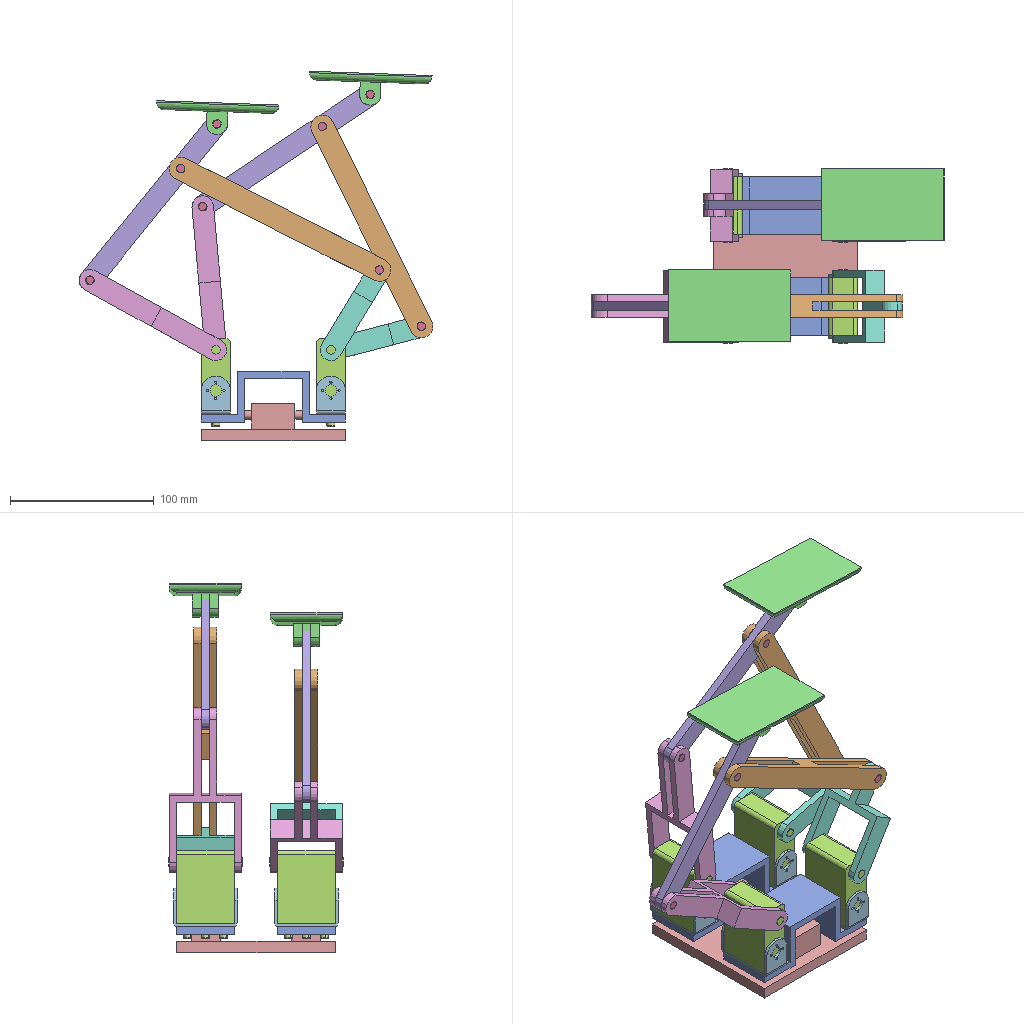Assembly | SolidWorks | 11 different items | 30 placed | box 246 x 121 x 257 mm
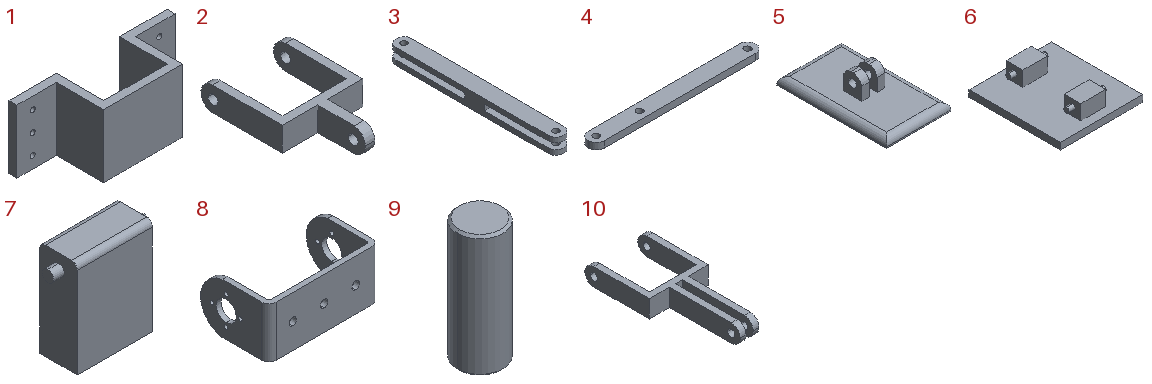Parts list (item | name | quantity | size | volume | features):
1 | - | x2 | 100 x 35 x 40 mm | 31788 mm3 | features Extrusion 1, ICE 1
2 | - | x2 | 50 x 80 x 15 mm | 12391 mm3 | features Extrusion 1, ICE 1
3 | - | x2 | 16 x 171 x 16 mm | 28165 mm3 | features Extrusion 1, ICE 1
4 | - | x2 | 155 x 15 x 6 mm | 13151 mm3 | features Extrusion 1
5 | - | x2 | 50 x 85 x 22 mm | 26297 mm3 | features ICE 3, Extrusion 1, Fillet 1
6 | - | x1 | 100 x 110 x 26 mm | 81963 mm3 | features ICE 3, Extrusion 1
7 | - | x4 | 51 x 20 x 51 mm | 40645 mm3 | features 3DProfileFeature 1, Extrusion 1, Fillet 1, HoleWzd 1, ICE 1
8 | - | x4 | 44 x 27 x 20 mm | 3261 mm3 | features ICE 2, Extrusion 1
9 | - | x8 | 6 x 6 x 16 mm | 450.749 mm3 | features Chamfer 1, Extrusion 1
10 | - | x2 | 50 x 115 x 15 mm | 19202 mm3 | features Extrusion 1, ICE 1
11 | hexagon socket head cap screws gb | x1 | - | - | -
Mates (type | each side: item.copy, entity, surface, feature):
Coincident | 6.1 face plane Boss-Extrude1 | 1.1 face plane Boss-Extrude1 | 2 times
Coincident | 1.1 face plane Boss-Extrude1 | 7.1 face plane Boss-Extrude1 | 2 times
Concentric | 7.1 face cylinder Boss-Extrude2 | 10.1 face cylinder Cut-Extrude1
Coincident | 7.1 face plane Boss-Extrude1 | 10.1 face plane Boss-Extrude1
Coincident | 1.1 face plane Boss-Extrude1 | 7.2 face plane Boss-Extrude1 | 2 times
Concentric | 2.1 face cylinder Cut-Extrude1 | 7.2 face cylinder Boss-Extrude2
Coincident | 2.1 face plane Boss-Extrude1 | 7.2 face plane Boss-Extrude1
DistanceDim | 1.1 face plane Boss-Extrude1 | 6.1 face plane Boss-Extrude1
Concentric | 2.1 face cylinder Cut-Extrude1 | 3.1 face cylinder Boss-Extrude1
Coincident | 2.1 face plane Boss-Extrude1 | 3.1 face plane Cut-Extrude1
Concentric | 10.1 face cylinder Cut-Extrude1 | 4.1 face cylinder Boss-Extrude1
Coincident | 10.1 face plane Boss-Extrude1 | 4.1 face plane Boss-Extrude1
Concentric | 3.1 face cylinder Boss-Extrude1 | 4.1 face cylinder Boss-Extrude1
Concentric | 4.1 face cylinder Boss-Extrude1 | 5.1 face cylinder Cut-Extrude2
Coincident | 4.1 face plane Boss-Extrude1 | 5.1 face plane Cut-Extrude1
Coincident | 1.2 face plane Boss-Extrude1 | 7.3 face plane Boss-Extrude1 | 2 times
Coincident | 1.1 face plane Boss-Extrude1 | 1.2 face plane Boss-Extrude1
Coincident | 6.1 face plane Boss-Extrude1 | 1.2 face plane Boss-Extrude1 | 2 times
Coincident | 7.4 face plane Boss-Extrude1 | 1.2 face plane Boss-Extrude1 | 2 times
Concentric | 10.2 face cylinder Cut-Extrude1 | 7.4 face cylinder Boss-Extrude2
Coincident | 10.2 face plane Boss-Extrude1 | 7.4 face plane Boss-Extrude1
Concentric | 4.2 face cylinder Boss-Extrude1 | 10.2 face cylinder Cut-Extrude1
Coincident | 4.2 face plane Boss-Extrude1 | 10.2 face plane Boss-Extrude1
Concentric | 3.2 face cylinder Boss-Extrude1 | 4.2 face cylinder Boss-Extrude1
Concentric | 2.2 face cylinder Cut-Extrude1 | 7.3 face cylinder Boss-Extrude2
Coincident | 2.2 face plane Boss-Extrude1 | 7.3 face plane Boss-Extrude1
Concentric | 3.2 face cylinder Boss-Extrude1 | 2.2 face cylinder Cut-Extrude1
Coincident | 3.2 face plane Cut-Extrude1 | 2.2 face plane Boss-Extrude1
Concentric | 5.2 face cylinder Cut-Extrude2 | 4.2 face cylinder Boss-Extrude1
Coincident | 5.2 face plane Cut-Extrude1 | 4.2 face plane Boss-Extrude1
Concentric | 5.2 face cylinder Cut-Extrude2 | 9.1 face cylinder Boss-Extrude1
Coincident | 5.2 face plane Boss-Extrude2 | 9.1 face plane Boss-Extrude1
Concentric | 3.2 face cylinder Boss-Extrude1 | 9.2 face cylinder Boss-Extrude1
Coincident | 3.2 face plane Boss-Extrude1 | 9.2 face plane Boss-Extrude1
Concentric | 10.2 face cylinder Cut-Extrude1 | 9.3 face cylinder Boss-Extrude1
Coincident | 10.2 face plane Boss-Extrude1 | 9.3 face plane Boss-Extrude1
Concentric | 10.1 face cylinder Cut-Extrude1 | 9.4 face cylinder Boss-Extrude1
Coincident | 10.1 face plane Boss-Extrude1 | 9.4 face plane Boss-Extrude1
Concentric | 3.1 face cylinder Boss-Extrude1 | 9.5 face cylinder Boss-Extrude1
Coincident | 3.1 face plane Boss-Extrude1 | 9.5 face plane Boss-Extrude1
Concentric | 3.2 face cylinder Boss-Extrude1 | 9.6 face cylinder Boss-Extrude1
Coincident | 3.2 face plane Boss-Extrude1 | 9.6 face plane Boss-Extrude1
Concentric | 3.1 face cylinder Boss-Extrude1 | 9.7 face cylinder Boss-Extrude1
Coincident | 3.1 face plane Boss-Extrude1 | 9.7 face plane Boss-Extrude1
Concentric | 5.1 face cylinder Cut-Extrude2 | 9.8 face cylinder Boss-Extrude1
Coincident | 5.1 face plane Boss-Extrude2 | 9.8 face plane Boss-Extrude1
Coincident | 7.4 face plane Boss-Extrude1 | 8.1 face plane Boss-Extrude1 | 3 times
Coincident | 7.1 face plane Boss-Extrude1 | 8.2 face plane Boss-Extrude1 | 3 times
Coincident | 7.2 face plane Boss-Extrude1 | 8.3 face plane Boss-Extrude1 | 3 times
Coincident | 7.3 face plane Boss-Extrude1 | 8.4 face plane Boss-Extrude1 | 3 times
Coincident | 1.1 face plane Boss-Extrude1 | 8.3 face plane Boss-Extrude1
Coincident | 1.2 face plane Boss-Extrude1 | 8.4 face plane Boss-Extrude1
Coincident | 1.1 face plane Boss-Extrude1 | 8.2 face plane Boss-Extrude1
Coincident | 1.2 face plane Boss-Extrude1 | 8.1 face plane Boss-Extrude1